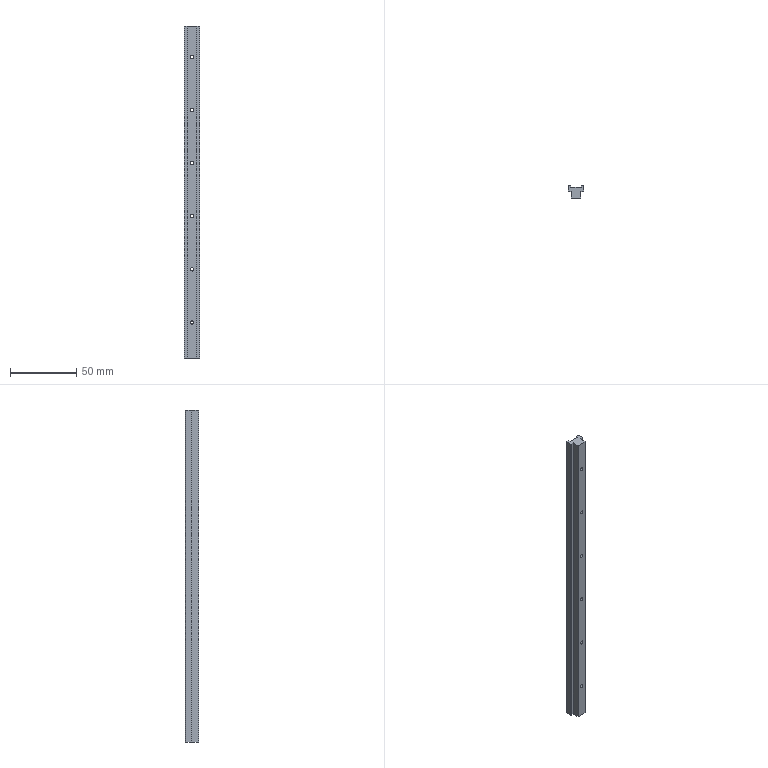Part | SolidWorks | features Chamfer 1, Extrusion 1, HoleWzd 1, LPattern 1 | 1 solid | 34 faces | box 12 x 10 x 250 mm | volume 20615 mm3 | plane 22 | cylinder 12 | commonest cylinder face diameters 2.5 x12
STEP:
#1=CARTESIAN_POINT('',(0.,-8.5,-59.5));
#2=VERTEX_POINT('',#1);
#3=CARTESIAN_POINT('',(0.,-8.5,-57.));
#4=VERTEX_POINT('',#3);
#5=CARTESIAN_POINT('',(0.,-8.5,-58.25));
#6=DIRECTION('',(0.,1.,0.));
#7=DIRECTION('',(0.,0.,1.));
#8=AXIS2_PLACEMENT_3D('',#5,#6,#7);
#9=CIRCLE('',#8,1.25);
#10=EDGE_CURVE('',#2,#4,#9,.T.);
#11=ORIENTED_EDGE('',*,*,#10,.F.);
#12=CARTESIAN_POINT('',(0.,0.,-59.5));
#13=VERTEX_POINT('',#12);
#14=CARTESIAN_POINT('',(0.,0.,-59.5));
#15=DIRECTION('',(0.,1.,0.));
#16=VECTOR('',#15,1000.);
#17=LINE('',#14,#16);
#18=EDGE_CURVE('',#2,#13,#17,.T.);
#19=ORIENTED_EDGE('',*,*,#18,.T.);
#20=CARTESIAN_POINT('',(0.,0.,-57.));
#21=VERTEX_POINT('',#20);
#22=CARTESIAN_POINT('',(0.,0.,-58.25));
#23=DIRECTION('',(0.,1.,0.));
#24=DIRECTION('',(0.,0.,1.));
#25=AXIS2_PLACEMENT_3D('',#22,#23,#24);
#26=CIRCLE('',#25,1.25);
#27=EDGE_CURVE('',#13,#21,#26,.T.);
#28=ORIENTED_EDGE('',*,*,#27,.T.);
#29=CARTESIAN_POINT('',(0.,0.,-57.));
#30=DIRECTION('',(0.,1.,0.));
#31=VECTOR('',#30,1000.);
#32=LINE('',#29,#31);
#33=EDGE_CURVE('',#4,#21,#32,.T.);
#34=ORIENTED_EDGE('',*,*,#33,.F.);
#35=EDGE_LOOP('',(#11,#19,#28,#34));
#36=FACE_OUTER_BOUND('',#35,.T.);
#37=CARTESIAN_POINT('',(0.,0.,-58.25));
#38=DIRECTION('',(0.,1.,0.));
#39=DIRECTION('',(0.,0.,1.));
#40=AXIS2_PLACEMENT_3D('',#37,#38,#39);
#41=CYLINDRICAL_SURFACE('',#40,1.25);
#42=ADVANCED_FACE('',(#36),#41,.F.);
#43=CARTESIAN_POINT('',(0.,-8.5,-99.5));
#44=VERTEX_POINT('',#43);
#45=CARTESIAN_POINT('',(0.,-8.5,-97.));
#46=VERTEX_POINT('',#45);
#47=CARTESIAN_POINT('',(0.,-8.5,-98.25));
#48=DIRECTION('',(0.,1.,0.));
#49=DIRECTION('',(0.,0.,1.));
#50=AXIS2_PLACEMENT_3D('',#47,#48,#49);
#51=CIRCLE('',#50,1.25);
#52=EDGE_CURVE('',#44,#46,#51,.T.);
#53=ORIENTED_EDGE('',*,*,#52,.F.);
#54=CARTESIAN_POINT('',(0.,0.,-99.5));
#55=VERTEX_POINT('',#54);
#56=CARTESIAN_POINT('',(0.,0.,-99.5));
#57=DIRECTION('',(0.,1.,0.));
#58=VECTOR('',#57,1000.);
#59=LINE('',#56,#58);
#60=EDGE_CURVE('',#44,#55,#59,.T.);
#61=ORIENTED_EDGE('',*,*,#60,.T.);
#62=CARTESIAN_POINT('',(0.,0.,-97.));
#63=VERTEX_POINT('',#62);
#64=CARTESIAN_POINT('',(0.,0.,-98.25));
#65=DIRECTION('',(0.,1.,0.));
#66=DIRECTION('',(0.,0.,1.));
#67=AXIS2_PLACEMENT_3D('',#64,#65,#66);
#68=CIRCLE('',#67,1.25);
#69=EDGE_CURVE('',#55,#63,#68,.T.);
#70=ORIENTED_EDGE('',*,*,#69,.T.);
#71=CARTESIAN_POINT('',(0.,0.,-97.));
#72=DIRECTION('',(0.,1.,0.));
#73=VECTOR('',#72,1000.);
#74=LINE('',#71,#73);
#75=EDGE_CURVE('',#46,#63,#74,.T.);
#76=ORIENTED_EDGE('',*,*,#75,.F.);
#77=EDGE_LOOP('',(#53,#61,#70,#76));
#78=FACE_OUTER_BOUND('',#77,.T.);
#79=CARTESIAN_POINT('',(0.,0.,-98.25));
#80=DIRECTION('',(0.,1.,0.));
#81=DIRECTION('',(0.,0.,1.));
#82=AXIS2_PLACEMENT_3D('',#79,#80,#81);
#83=CYLINDRICAL_SURFACE('',#82,1.25);
#84=ADVANCED_FACE('',(#78),#83,.F.);
#85=CARTESIAN_POINT('',(0.,-8.5,-19.5));
#86=VERTEX_POINT('',#85);
#87=CARTESIAN_POINT('',(0.,-8.5,-17.));
#88=VERTEX_POINT('',#87);
#89=CARTESIAN_POINT('',(0.,-8.5,-18.25));
#90=DIRECTION('',(0.,1.,0.));
#91=DIRECTION('',(0.,0.,1.));
#92=AXIS2_PLACEMENT_3D('',#89,#90,#91);
#93=CIRCLE('',#92,1.25);
#94=EDGE_CURVE('',#86,#88,#93,.T.);
#95=ORIENTED_EDGE('',*,*,#94,.F.);
#96=CARTESIAN_POINT('',(0.,0.,-19.5));
#97=VERTEX_POINT('',#96);
#98=CARTESIAN_POINT('',(0.,0.,-19.5));
#99=DIRECTION('',(0.,1.,0.));
#100=VECTOR('',#99,1000.);
#101=LINE('',#98,#100);
#102=EDGE_CURVE('',#86,#97,#101,.T.);
#103=ORIENTED_EDGE('',*,*,#102,.T.);
#104=CARTESIAN_POINT('',(0.,0.,-17.));
#105=VERTEX_POINT('',#104);
#106=CARTESIAN_POINT('',(0.,0.,-18.25));
#107=DIRECTION('',(0.,1.,0.));
#108=DIRECTION('',(0.,0.,1.));
#109=AXIS2_PLACEMENT_3D('',#106,#107,#108);
#110=CIRCLE('',#109,1.25);
#111=EDGE_CURVE('',#97,#105,#110,.T.);
#112=ORIENTED_EDGE('',*,*,#111,.T.);
#113=CARTESIAN_POINT('',(0.,0.,-17.));
#114=DIRECTION('',(0.,1.,0.));
#115=VECTOR('',#114,1000.);
#116=LINE('',#113,#115);
#117=EDGE_CURVE('',#88,#105,#116,.T.);
#118=ORIENTED_EDGE('',*,*,#117,.F.);
#119=EDGE_LOOP('',(#95,#103,#112,#118));
#120=FACE_OUTER_BOUND('',#119,.T.);
#121=CARTESIAN_POINT('',(0.,0.,-18.25));
#122=DIRECTION('',(0.,1.,0.));
#123=DIRECTION('',(0.,0.,1.));
#124=AXIS2_PLACEMENT_3D('',#121,#122,#123);
#125=CYLINDRICAL_SURFACE('',#124,1.25);
#126=ADVANCED_FACE('',(#120),#125,.F.);
#127=CARTESIAN_POINT('',(0.,-8.5,20.5));
#128=VERTEX_POINT('',#127);
#129=CARTESIAN_POINT('',(0.,-8.5,23.));
#130=VERTEX_POINT('',#129);
#131=CARTESIAN_POINT('',(0.,-8.5,21.75));
#132=DIRECTION('',(0.,1.,0.));
#133=DIRECTION('',(0.,0.,1.));
#134=AXIS2_PLACEMENT_3D('',#131,#132,#133);
#135=CIRCLE('',#134,1.25);
#136=EDGE_CURVE('',#128,#130,#135,.T.);
#137=ORIENTED_EDGE('',*,*,#136,.F.);
#138=CARTESIAN_POINT('',(0.,0.,20.5));
#139=VERTEX_POINT('',#138);
#140=CARTESIAN_POINT('',(0.,0.,20.5));
#141=DIRECTION('',(0.,1.,0.));
#142=VECTOR('',#141,1000.);
#143=LINE('',#140,#142);
#144=EDGE_CURVE('',#128,#139,#143,.T.);
#145=ORIENTED_EDGE('',*,*,#144,.T.);
#146=CARTESIAN_POINT('',(0.,0.,23.));
#147=VERTEX_POINT('',#146);
#148=CARTESIAN_POINT('',(0.,0.,21.75));
#149=DIRECTION('',(0.,1.,0.));
#150=DIRECTION('',(0.,0.,1.));
#151=AXIS2_PLACEMENT_3D('',#148,#149,#150);
#152=CIRCLE('',#151,1.25);
#153=EDGE_CURVE('',#139,#147,#152,.T.);
#154=ORIENTED_EDGE('',*,*,#153,.T.);
#155=CARTESIAN_POINT('',(0.,0.,23.));
#156=DIRECTION('',(0.,1.,0.));
#157=VECTOR('',#156,1000.);
#158=LINE('',#155,#157);
#159=EDGE_CURVE('',#130,#147,#158,.T.);
#160=ORIENTED_EDGE('',*,*,#159,.F.);
#161=EDGE_LOOP('',(#137,#145,#154,#160));
#162=FACE_OUTER_BOUND('',#161,.T.);
#163=CARTESIAN_POINT('',(0.,0.,21.75));
#164=DIRECTION('',(0.,1.,0.));
#165=DIRECTION('',(0.,0.,1.));
#166=AXIS2_PLACEMENT_3D('',#163,#164,#165);
#167=CYLINDRICAL_SURFACE('',#166,1.25);
#168=ADVANCED_FACE('',(#162),#167,.F.);
#169=CARTESIAN_POINT('',(0.,-8.5,60.5));
#170=VERTEX_POINT('',#169);
#171=CARTESIAN_POINT('',(0.,-8.5,63.));
#172=VERTEX_POINT('',#171);
#173=CARTESIAN_POINT('',(0.,-8.5,61.75));
#174=DIRECTION('',(0.,1.,0.));
#175=DIRECTION('',(0.,0.,1.));
#176=AXIS2_PLACEMENT_3D('',#173,#174,#175);
#177=CIRCLE('',#176,1.25);
#178=EDGE_CURVE('',#170,#172,#177,.T.);
#179=ORIENTED_EDGE('',*,*,#178,.F.);
#180=CARTESIAN_POINT('',(0.,0.,60.5));
#181=VERTEX_POINT('',#180);
#182=CARTESIAN_POINT('',(0.,0.,60.5));
#183=DIRECTION('',(0.,1.,0.));
#184=VECTOR('',#183,1000.);
#185=LINE('',#182,#184);
#186=EDGE_CURVE('',#170,#181,#185,.T.);
#187=ORIENTED_EDGE('',*,*,#186,.T.);
#188=CARTESIAN_POINT('',(0.,0.,63.));
#189=VERTEX_POINT('',#188);
#190=CARTESIAN_POINT('',(0.,0.,61.75));
#191=DIRECTION('',(0.,1.,0.));
#192=DIRECTION('',(0.,0.,1.));
#193=AXIS2_PLACEMENT_3D('',#190,#191,#192);
#194=CIRCLE('',#193,1.25);
#195=EDGE_CURVE('',#181,#189,#194,.T.);
#196=ORIENTED_EDGE('',*,*,#195,.T.);
#197=CARTESIAN_POINT('',(0.,0.,63.));
#198=DIRECTION('',(0.,1.,0.));
#199=VECTOR('',#198,1000.);
#200=LINE('',#197,#199);
#201=EDGE_CURVE('',#172,#189,#200,.T.);
#202=ORIENTED_EDGE('',*,*,#201,.F.);
#203=EDGE_LOOP('',(#179,#187,#196,#202));
#204=FACE_OUTER_BOUND('',#203,.T.);
#205=CARTESIAN_POINT('',(0.,0.,61.75));
#206=DIRECTION('',(0.,1.,0.));
#207=DIRECTION('',(0.,0.,1.));
#208=AXIS2_PLACEMENT_3D('',#205,#206,#207);
#209=CYLINDRICAL_SURFACE('',#208,1.25);
#210=ADVANCED_FACE('',(#204),#209,.F.);
#211=CARTESIAN_POINT('',(0.,-8.5,100.5));
#212=VERTEX_POINT('',#211);
#213=CARTESIAN_POINT('',(0.,-8.5,103.));
#214=VERTEX_POINT('',#213);
#215=CARTESIAN_POINT('',(0.,-8.5,101.75));
#216=DIRECTION('',(0.,1.,0.));
#217=DIRECTION('',(0.,0.,1.));
#218=AXIS2_PLACEMENT_3D('',#215,#216,#217);
#219=CIRCLE('',#218,1.25);
#220=EDGE_CURVE('',#212,#214,#219,.T.);
#221=ORIENTED_EDGE('',*,*,#220,.F.);
#222=CARTESIAN_POINT('',(0.,0.,100.5));
#223=VERTEX_POINT('',#222);
#224=CARTESIAN_POINT('',(0.,0.,100.5));
#225=DIRECTION('',(0.,1.,0.));
#226=VECTOR('',#225,1000.);
#227=LINE('',#224,#226);
#228=EDGE_CURVE('',#212,#223,#227,.T.);
#229=ORIENTED_EDGE('',*,*,#228,.T.);
#230=CARTESIAN_POINT('',(0.,0.,103.));
#231=VERTEX_POINT('',#230);
#232=CARTESIAN_POINT('',(0.,0.,101.75));
#233=DIRECTION('',(0.,1.,0.));
#234=DIRECTION('',(0.,0.,1.));
#235=AXIS2_PLACEMENT_3D('',#232,#233,#234);
#236=CIRCLE('',#235,1.25);
#237=EDGE_CURVE('',#223,#231,#236,.T.);
#238=ORIENTED_EDGE('',*,*,#237,.T.);
#239=CARTESIAN_POINT('',(0.,0.,103.));
#240=DIRECTION('',(0.,1.,0.));
#241=VECTOR('',#240,1000.);
#242=LINE('',#239,#241);
#243=EDGE_CURVE('',#214,#231,#242,.T.);
#244=ORIENTED_EDGE('',*,*,#243,.F.);
#245=EDGE_LOOP('',(#221,#229,#238,#244));
#246=FACE_OUTER_BOUND('',#245,.T.);
#247=CARTESIAN_POINT('',(0.,0.,101.75));
#248=DIRECTION('',(0.,1.,0.));
#249=DIRECTION('',(0.,0.,1.));
#250=AXIS2_PLACEMENT_3D('',#247,#248,#249);
#251=CYLINDRICAL_SURFACE('',#250,1.25);
#252=ADVANCED_FACE('',(#246),#251,.F.);
#253=ORIENTED_EDGE('',*,*,#228,.F.);
#254=CARTESIAN_POINT('',(0.,-8.5,101.75));
#255=DIRECTION('',(0.,1.,0.));
#256=DIRECTION('',(0.,0.,1.));
#257=AXIS2_PLACEMENT_3D('',#254,#255,#256);
#258=CIRCLE('',#257,1.25);
#259=EDGE_CURVE('',#214,#212,#258,.T.);
#260=ORIENTED_EDGE('',*,*,#259,.F.);
#261=ORIENTED_EDGE('',*,*,#243,.T.);
#262=CARTESIAN_POINT('',(0.,0.,101.75));
#263=DIRECTION('',(0.,1.,0.));
#264=DIRECTION('',(0.,0.,1.));
#265=AXIS2_PLACEMENT_3D('',#262,#263,#264);
#266=CIRCLE('',#265,1.25);
#267=EDGE_CURVE('',#231,#223,#266,.T.);
#268=ORIENTED_EDGE('',*,*,#267,.T.);
#269=EDGE_LOOP('',(#253,#260,#261,#268));
#270=FACE_OUTER_BOUND('',#269,.T.);
#271=CARTESIAN_POINT('',(0.,0.,101.75));
#272=DIRECTION('',(0.,1.,0.));
#273=DIRECTION('',(0.,0.,1.));
#274=AXIS2_PLACEMENT_3D('',#271,#272,#273);
#275=CYLINDRICAL_SURFACE('',#274,1.25);
#276=ADVANCED_FACE('',(#270),#275,.F.);
#277=ORIENTED_EDGE('',*,*,#186,.F.);
#278=CARTESIAN_POINT('',(0.,-8.5,61.75));
#279=DIRECTION('',(0.,1.,0.));
#280=DIRECTION('',(0.,0.,1.));
#281=AXIS2_PLACEMENT_3D('',#278,#279,#280);
#282=CIRCLE('',#281,1.25);
#283=EDGE_CURVE('',#172,#170,#282,.T.);
#284=ORIENTED_EDGE('',*,*,#283,.F.);
#285=ORIENTED_EDGE('',*,*,#201,.T.);
#286=CARTESIAN_POINT('',(0.,0.,61.75));
#287=DIRECTION('',(0.,1.,0.));
#288=DIRECTION('',(0.,0.,1.));
#289=AXIS2_PLACEMENT_3D('',#286,#287,#288);
#290=CIRCLE('',#289,1.25);
#291=EDGE_CURVE('',#189,#181,#290,.T.);
#292=ORIENTED_EDGE('',*,*,#291,.T.);
#293=EDGE_LOOP('',(#277,#284,#285,#292));
#294=FACE_OUTER_BOUND('',#293,.T.);
#295=CARTESIAN_POINT('',(0.,0.,61.75));
#296=DIRECTION('',(0.,1.,0.));
#297=DIRECTION('',(0.,0.,1.));
#298=AXIS2_PLACEMENT_3D('',#295,#296,#297);
#299=CYLINDRICAL_SURFACE('',#298,1.25);
#300=ADVANCED_FACE('',(#294),#299,.F.);
#301=ORIENTED_EDGE('',*,*,#144,.F.);
#302=CARTESIAN_POINT('',(0.,-8.5,21.75));
#303=DIRECTION('',(0.,1.,0.));
#304=DIRECTION('',(0.,0.,1.));
#305=AXIS2_PLACEMENT_3D('',#302,#303,#304);
#306=CIRCLE('',#305,1.25);
#307=EDGE_CURVE('',#130,#128,#306,.T.);
#308=ORIENTED_EDGE('',*,*,#307,.F.);
#309=ORIENTED_EDGE('',*,*,#159,.T.);
#310=CARTESIAN_POINT('',(0.,0.,21.75));
#311=DIRECTION('',(0.,1.,0.));
#312=DIRECTION('',(0.,0.,1.));
#313=AXIS2_PLACEMENT_3D('',#310,#311,#312);
#314=CIRCLE('',#313,1.25);
#315=EDGE_CURVE('',#147,#139,#314,.T.);
#316=ORIENTED_EDGE('',*,*,#315,.T.);
#317=EDGE_LOOP('',(#301,#308,#309,#316));
#318=FACE_OUTER_BOUND('',#317,.T.);
#319=CARTESIAN_POINT('',(0.,0.,21.75));
#320=DIRECTION('',(0.,1.,0.));
#321=DIRECTION('',(0.,0.,1.));
#322=AXIS2_PLACEMENT_3D('',#319,#320,#321);
#323=CYLINDRICAL_SURFACE('',#322,1.25);
#324=ADVANCED_FACE('',(#318),#323,.F.);
#325=ORIENTED_EDGE('',*,*,#102,.F.);
#326=CARTESIAN_POINT('',(0.,-8.5,-18.25));
#327=DIRECTION('',(0.,1.,0.));
#328=DIRECTION('',(0.,0.,1.));
#329=AXIS2_PLACEMENT_3D('',#326,#327,#328);
#330=CIRCLE('',#329,1.25);
#331=EDGE_CURVE('',#88,#86,#330,.T.);
#332=ORIENTED_EDGE('',*,*,#331,.F.);
#333=ORIENTED_EDGE('',*,*,#117,.T.);
#334=CARTESIAN_POINT('',(0.,0.,-18.25));
#335=DIRECTION('',(0.,1.,0.));
#336=DIRECTION('',(0.,0.,1.));
#337=AXIS2_PLACEMENT_3D('',#334,#335,#336);
#338=CIRCLE('',#337,1.25);
#339=EDGE_CURVE('',#105,#97,#338,.T.);
#340=ORIENTED_EDGE('',*,*,#339,.T.);
#341=EDGE_LOOP('',(#325,#332,#333,#340));
#342=FACE_OUTER_BOUND('',#341,.T.);
#343=CARTESIAN_POINT('',(0.,0.,-18.25));
#344=DIRECTION('',(0.,1.,0.));
#345=DIRECTION('',(0.,0.,1.));
#346=AXIS2_PLACEMENT_3D('',#343,#344,#345);
#347=CYLINDRICAL_SURFACE('',#346,1.25);
#348=ADVANCED_FACE('',(#342),#347,.F.);
#349=CARTESIAN_POINT('',(-4.,0.,-125.));
#350=VERTEX_POINT('',#349);
#351=CARTESIAN_POINT('',(-4.,1.3,-125.));
#352=VERTEX_POINT('',#351);
#353=CARTESIAN_POINT('',(-4.,0.,-125.));
#354=DIRECTION('',(0.,1.,0.));
#355=VECTOR('',#354,1000.);
#356=LINE('',#353,#355);
#357=EDGE_CURVE('',#350,#352,#356,.T.);
#358=ORIENTED_EDGE('',*,*,#357,.T.);
#359=CARTESIAN_POINT('',(-4.,1.3,125.));
#360=VERTEX_POINT('',#359);
#361=CARTESIAN_POINT('',(-4.,1.3,125.));
#362=DIRECTION('',(0.,0.,1.));
#363=VECTOR('',#362,1000.);
#364=LINE('',#361,#363);
#365=EDGE_CURVE('',#352,#360,#364,.T.);
#366=ORIENTED_EDGE('',*,*,#365,.T.);
#367=CARTESIAN_POINT('',(-4.,0.,125.));
#368=VERTEX_POINT('',#367);
#369=CARTESIAN_POINT('',(-4.,0.,125.));
#370=DIRECTION('',(0.,1.,0.));
#371=VECTOR('',#370,1000.);
#372=LINE('',#369,#371);
#373=EDGE_CURVE('',#368,#360,#372,.T.);
#374=ORIENTED_EDGE('',*,*,#373,.F.);
#375=CARTESIAN_POINT('',(-4.,0.,125.));
#376=DIRECTION('',(0.,0.,-1.));
#377=VECTOR('',#376,1000.);
#378=LINE('',#375,#377);
#379=EDGE_CURVE('',#368,#350,#378,.T.);
#380=ORIENTED_EDGE('',*,*,#379,.T.);
#381=EDGE_LOOP('',(#358,#366,#374,#380));
#382=FACE_OUTER_BOUND('',#381,.T.);
#383=CARTESIAN_POINT('',(-4.,0.,125.));
#384=DIRECTION('',(-1.,0.,0.));
#385=DIRECTION('',(0.,-1.,0.));
#386=AXIS2_PLACEMENT_3D('',#383,#384,#385);
#387=PLANE('',#386);
#388=ADVANCED_FACE('',(#382),#387,.F.);
#389=CARTESIAN_POINT('',(-4.2,1.5,-125.));
#390=VERTEX_POINT('',#389);
#391=CARTESIAN_POINT('',(-5.8,1.5,-125.));
#392=VERTEX_POINT('',#391);
#393=CARTESIAN_POINT('',(-4.,1.5,-125.));
#394=DIRECTION('',(-1.,0.,0.));
#395=VECTOR('',#394,1000.);
#396=LINE('',#393,#395);
#397=EDGE_CURVE('',#390,#392,#396,.T.);
#398=ORIENTED_EDGE('',*,*,#397,.T.);
#399=CARTESIAN_POINT('',(-5.8,1.5,125.));
#400=VERTEX_POINT('',#399);
#401=CARTESIAN_POINT('',(-5.8,1.5,125.));
#402=DIRECTION('',(0.,0.,1.));
#403=VECTOR('',#402,1000.);
#404=LINE('',#401,#403);
#405=EDGE_CURVE('',#392,#400,#404,.T.);
#406=ORIENTED_EDGE('',*,*,#405,.T.);
#407=CARTESIAN_POINT('',(-4.2,1.5,125.));
#408=VERTEX_POINT('',#407);
#409=CARTESIAN_POINT('',(-4.,1.5,125.));
#410=DIRECTION('',(-1.,0.,0.));
#411=VECTOR('',#410,1000.);
#412=LINE('',#409,#411);
#413=EDGE_CURVE('',#408,#400,#412,.T.);
#414=ORIENTED_EDGE('',*,*,#413,.F.);
#415=CARTESIAN_POINT('',(-4.2,1.5,125.));
#416=DIRECTION('',(0.,0.,-1.));
#417=VECTOR('',#416,1000.);
#418=LINE('',#415,#417);
#419=EDGE_CURVE('',#408,#390,#418,.T.);
#420=ORIENTED_EDGE('',*,*,#419,.T.);
#421=EDGE_LOOP('',(#398,#406,#414,#420));
#422=FACE_OUTER_BOUND('',#421,.T.);
#423=CARTESIAN_POINT('',(-4.,1.5,125.));
#424=DIRECTION('',(0.,-1.,0.));
#425=DIRECTION('',(0.,0.,-1.));
#426=AXIS2_PLACEMENT_3D('',#423,#424,#425);
#427=PLANE('',#426);
#428=ADVANCED_FACE('',(#422),#427,.F.);
#429=CARTESIAN_POINT('',(-6.,1.3,125.));
#430=VERTEX_POINT('',#429);
#431=CARTESIAN_POINT('',(-6.,-3.,125.));
#432=VERTEX_POINT('',#431);
#433=CARTESIAN_POINT('',(-6.,1.5,125.));
#434=DIRECTION('',(0.,-1.,0.));
#435=VECTOR('',#434,1000.);
#436=LINE('',#433,#435);
#437=EDGE_CURVE('',#430,#432,#436,.T.);
#438=ORIENTED_EDGE('',*,*,#437,.F.);
#439=CARTESIAN_POINT('',(-6.,1.3,-125.));
#440=VERTEX_POINT('',#439);
#441=CARTESIAN_POINT('',(-6.,1.3,125.));
#442=DIRECTION('',(0.,0.,-1.));
#443=VECTOR('',#442,1000.);
#444=LINE('',#441,#443);
#445=EDGE_CURVE('',#430,#440,#444,.T.);
#446=ORIENTED_EDGE('',*,*,#445,.T.);
#447=CARTESIAN_POINT('',(-6.,-3.,-125.));
#448=VERTEX_POINT('',#447);
#449=CARTESIAN_POINT('',(-6.,1.5,-125.));
#450=DIRECTION('',(0.,-1.,0.));
#451=VECTOR('',#450,1000.);
#452=LINE('',#449,#451);
#453=EDGE_CURVE('',#440,#448,#452,.T.);
#454=ORIENTED_EDGE('',*,*,#453,.T.);
#455=CARTESIAN_POINT('',(-6.,-3.,125.));
#456=DIRECTION('',(0.,0.,1.));
#457=VECTOR('',#456,1000.);
#458=LINE('',#455,#457);
#459=EDGE_CURVE('',#448,#432,#458,.T.);
#460=ORIENTED_EDGE('',*,*,#459,.T.);
#461=EDGE_LOOP('',(#438,#446,#454,#460));
#462=FACE_OUTER_BOUND('',#461,.T.);
#463=CARTESIAN_POINT('',(-6.,1.5,125.));
#464=DIRECTION('',(1.,0.,0.));
#465=DIRECTION('',(0.,1.,0.));
#466=AXIS2_PLACEMENT_3D('',#463,#464,#465);
#467=PLANE('',#466);
#468=ADVANCED_FACE('',(#462),#467,.F.);
#469=CARTESIAN_POINT('',(-5.8,-3.2,125.));
#470=VERTEX_POINT('',#469);
#471=CARTESIAN_POINT('',(-3.7,-3.2,125.));
#472=VERTEX_POINT('',#471);
#473=CARTESIAN_POINT('',(-6.,-3.2,125.));
#474=DIRECTION('',(1.,0.,0.));
#475=VECTOR('',#474,1000.);
#476=LINE('',#473,#475);
#477=EDGE_CURVE('',#470,#472,#476,.T.);
#478=ORIENTED_EDGE('',*,*,#477,.F.);
#479=CARTESIAN_POINT('',(-5.8,-3.2,-125.));
#480=VERTEX_POINT('',#479);
#481=CARTESIAN_POINT('',(-5.8,-3.2,125.));
#482=DIRECTION('',(0.,0.,-1.));
#483=VECTOR('',#482,1000.);
#484=LINE('',#481,#483);
#485=EDGE_CURVE('',#470,#480,#484,.T.);
#486=ORIENTED_EDGE('',*,*,#485,.T.);
#487=CARTESIAN_POINT('',(-3.7,-3.2,-125.));
#488=VERTEX_POINT('',#487);
#489=CARTESIAN_POINT('',(-6.,-3.2,-125.));
#490=DIRECTION('',(1.,0.,0.));
#491=VECTOR('',#490,1000.);
#492=LINE('',#489,#491);
#493=EDGE_CURVE('',#480,#488,#492,.T.);
#494=ORIENTED_EDGE('',*,*,#493,.T.);
#495=CARTESIAN_POINT('',(-3.7,-3.2,125.));
#496=DIRECTION('',(0.,0.,-1.));
#497=VECTOR('',#496,1000.);
#498=LINE('',#495,#497);
#499=EDGE_CURVE('',#472,#488,#498,.T.);
#500=ORIENTED_EDGE('',*,*,#499,.F.);
#501=EDGE_LOOP('',(#478,#486,#494,#500));
#502=FACE_OUTER_BOUND('',#501,.T.);
#503=CARTESIAN_POINT('',(-6.,-3.2,125.));
#504=DIRECTION('',(0.,1.,0.));
#505=DIRECTION('',(0.,0.,1.));
#506=AXIS2_PLACEMENT_3D('',#503,#504,#505);
#507=PLANE('',#506);
#508=ADVANCED_FACE('',(#502),#507,.F.);
#509=CARTESIAN_POINT('',(-3.7,-8.3,-125.));
#510=VERTEX_POINT('',#509);
#511=CARTESIAN_POINT('',(-3.7,-3.2,-125.));
#512=DIRECTION('',(0.,-1.,0.));
#513=VECTOR('',#512,1000.);
#514=LINE('',#511,#513);
#515=EDGE_CURVE('',#488,#510,#514,.T.);
#516=ORIENTED_EDGE('',*,*,#515,.T.);
#517=CARTESIAN_POINT('',(-3.7,-8.3,125.));
#518=VERTEX_POINT('',#517);
#519=CARTESIAN_POINT('',(-3.7,-8.3,125.));
#520=DIRECTION('',(0.,0.,1.));
#521=VECTOR('',#520,1000.);
#522=LINE('',#519,#521);
#523=EDGE_CURVE('',#510,#518,#522,.T.);
#524=ORIENTED_EDGE('',*,*,#523,.T.);
#525=CARTESIAN_POINT('',(-3.7,-3.2,125.));
#526=DIRECTION('',(0.,-1.,0.));
#527=VECTOR('',#526,1000.);
#528=LINE('',#525,#527);
#529=EDGE_CURVE('',#472,#518,#528,.T.);
#530=ORIENTED_EDGE('',*,*,#529,.F.);
#531=ORIENTED_EDGE('',*,*,#499,.T.);
#532=EDGE_LOOP('',(#516,#524,#530,#531));
#533=FACE_OUTER_BOUND('',#532,.T.);
#534=CARTESIAN_POINT('',(-3.7,-3.2,125.));
#535=DIRECTION('',(1.,0.,0.));
#536=DIRECTION('',(0.,1.,0.));
#537=AXIS2_PLACEMENT_3D('',#534,#535,#536);
#538=PLANE('',#537);
#539=ADVANCED_FACE('',(#533),#538,.F.);
#540=CARTESIAN_POINT('',(0.,-8.5,-58.25));
#541=DIRECTION('',(0.,1.,0.));
#542=DIRECTION('',(0.,0.,1.));
#543=AXIS2_PLACEMENT_3D('',#540,#541,#542);
#544=CIRCLE('',#543,1.25);
#545=EDGE_CURVE('',#4,#2,#544,.T.);
#546=ORIENTED_EDGE('',*,*,#545,.T.);
#547=ORIENTED_EDGE('',*,*,#10,.T.);
#548=EDGE_LOOP('',(#546,#547));
#549=FACE_BOUND('',#548,.T.);
#550=CARTESIAN_POINT('',(0.,-8.5,-98.25));
#551=DIRECTION('',(0.,1.,0.));
#552=DIRECTION('',(0.,0.,1.));
#553=AXIS2_PLACEMENT_3D('',#550,#551,#552);
#554=CIRCLE('',#553,1.25);
#555=EDGE_CURVE('',#46,#44,#554,.T.);
#556=ORIENTED_EDGE('',*,*,#555,.T.);
#557=ORIENTED_EDGE('',*,*,#52,.T.);
#558=EDGE_LOOP('',(#556,#557));
#559=FACE_BOUND('',#558,.T.);
#560=CARTESIAN_POINT('',(-3.5,-8.5,125.));
#561=VERTEX_POINT('',#560);
#562=CARTESIAN_POINT('',(3.5,-8.5,125.));
#563=VERTEX_POINT('',#562);
#564=CARTESIAN_POINT('',(-3.7,-8.5,125.));
#565=DIRECTION('',(1.,0.,0.));
#566=VECTOR('',#565,1000.);
#567=LINE('',#564,#566);
#568=EDGE_CURVE('',#561,#563,#567,.T.);
#569=ORIENTED_EDGE('',*,*,#568,.F.);
#570=CARTESIAN_POINT('',(-3.5,-8.5,-125.));
#571=VERTEX_POINT('',#570);
#572=CARTESIAN_POINT('',(-3.5,-8.5,125.));
#573=DIRECTION('',(0.,0.,-1.));
#574=VECTOR('',#573,1000.);
#575=LINE('',#572,#574);
#576=EDGE_CURVE('',#561,#571,#575,.T.);
#577=ORIENTED_EDGE('',*,*,#576,.T.);
#578=CARTESIAN_POINT('',(3.5,-8.5,-125.));
#579=VERTEX_POINT('',#578);
#580=CARTESIAN_POINT('',(-3.7,-8.5,-125.));
#581=DIRECTION('',(1.,0.,0.));
#582=VECTOR('',#581,1000.);
#583=LINE('',#580,#582);
#584=EDGE_CURVE('',#571,#579,#583,.T.);
#585=ORIENTED_EDGE('',*,*,#584,.T.);
#586=CARTESIAN_POINT('',(3.5,-8.5,125.));
#587=DIRECTION('',(0.,0.,1.));
#588=VECTOR('',#587,1000.);
#589=LINE('',#586,#588);
#590=EDGE_CURVE('',#579,#563,#589,.T.);
#591=ORIENTED_EDGE('',*,*,#590,.T.);
#592=EDGE_LOOP('',(#569,#577,#585,#591));
#593=FACE_OUTER_BOUND('',#592,.T.);
#594=ORIENTED_EDGE('',*,*,#331,.T.);
#595=ORIENTED_EDGE('',*,*,#94,.T.);
#596=EDGE_LOOP('',(#594,#595));
#597=FACE_BOUND('',#596,.T.);
#598=ORIENTED_EDGE('',*,*,#307,.T.);
#599=ORIENTED_EDGE('',*,*,#136,.T.);
#600=EDGE_LOOP('',(#598,#599));
#601=FACE_BOUND('',#600,.T.);
#602=ORIENTED_EDGE('',*,*,#283,.T.);
#603=ORIENTED_EDGE('',*,*,#178,.T.);
#604=EDGE_LOOP('',(#602,#603));
#605=FACE_BOUND('',#604,.T.);
#606=ORIENTED_EDGE('',*,*,#259,.T.);
#607=ORIENTED_EDGE('',*,*,#220,.T.);
#608=EDGE_LOOP('',(#606,#607));
#609=FACE_BOUND('',#608,.T.);
#610=CARTESIAN_POINT('',(-3.7,-8.5,125.));
#611=DIRECTION('',(0.,1.,0.));
#612=DIRECTION('',(0.,0.,1.));
#613=AXIS2_PLACEMENT_3D('',#610,#611,#612);
#614=PLANE('',#613);
#615=ADVANCED_FACE('',(#549,#559,#593,#597,#601,#605,#609),#614,.F.);
#616=CARTESIAN_POINT('',(3.7,-8.3,125.));
#617=VERTEX_POINT('',#616);
#618=CARTESIAN_POINT('',(3.7,-3.2,125.));
#619=VERTEX_POINT('',#618);
#620=CARTESIAN_POINT('',(3.7,-3.2,125.));
#621=DIRECTION('',(0.,1.,0.));
#622=VECTOR('',#621,1000.);
#623=LINE('',#620,#622);
#624=EDGE_CURVE('',#617,#619,#623,.T.);
#625=ORIENTED_EDGE('',*,*,#624,.F.);
#626=CARTESIAN_POINT('',(3.7,-8.3,-125.));
#627=VERTEX_POINT('',#626);
#628=CARTESIAN_POINT('',(3.7,-8.3,125.));
#629=DIRECTION('',(0.,0.,-1.));
#630=VECTOR('',#629,1000.);
#631=LINE('',#628,#630);
#632=EDGE_CURVE('',#617,#627,#631,.T.);
#633=ORIENTED_EDGE('',*,*,#632,.T.);
#634=CARTESIAN_POINT('',(3.7,-3.2,-125.));
#635=VERTEX_POINT('',#634);
#636=CARTESIAN_POINT('',(3.7,-3.2,-125.));
#637=DIRECTION('',(0.,1.,0.));
#638=VECTOR('',#637,1000.);
#639=LINE('',#636,#638);
#640=EDGE_CURVE('',#627,#635,#639,.T.);
#641=ORIENTED_EDGE('',*,*,#640,.T.);
#642=CARTESIAN_POINT('',(3.7,-3.2,125.));
#643=DIRECTION('',(0.,0.,-1.));
#644=VECTOR('',#643,1000.);
#645=LINE('',#642,#644);
#646=EDGE_CURVE('',#619,#635,#645,.T.);
#647=ORIENTED_EDGE('',*,*,#646,.F.);
#648=EDGE_LOOP('',(#625,#633,#641,#647));
#649=FACE_OUTER_BOUND('',#648,.T.);
#650=CARTESIAN_POINT('',(3.7,-3.2,125.));
#651=DIRECTION('',(-1.,0.,0.));
#652=DIRECTION('',(0.,-1.,0.));
#653=AXIS2_PLACEMENT_3D('',#650,#651,#652);
#654=PLANE('',#653);
#655=ADVANCED_FACE('',(#649),#654,.F.);
#656=CARTESIAN_POINT('',(5.8,-3.2,-125.));
#657=VERTEX_POINT('',#656);
#658=CARTESIAN_POINT('',(6.,-3.2,-125.));
#659=DIRECTION('',(1.,0.,0.));
#660=VECTOR('',#659,1000.);
#661=LINE('',#658,#660);
#662=EDGE_CURVE('',#635,#657,#661,.T.);
#663=ORIENTED_EDGE('',*,*,#662,.T.);
#664=CARTESIAN_POINT('',(5.8,-3.2,125.));
#665=VERTEX_POINT('',#664);
#666=CARTESIAN_POINT('',(5.8,-3.2,125.));
#667=DIRECTION('',(0.,0.,1.));
#668=VECTOR('',#667,1000.);
#669=LINE('',#666,#668);
#670=EDGE_CURVE('',#657,#665,#669,.T.);
#671=ORIENTED_EDGE('',*,*,#670,.T.);
#672=CARTESIAN_POINT('',(6.,-3.2,125.));
#673=DIRECTION('',(1.,0.,0.));
#674=VECTOR('',#673,1000.);
#675=LINE('',#672,#674);
#676=EDGE_CURVE('',#619,#665,#675,.T.);
#677=ORIENTED_EDGE('',*,*,#676,.F.);
#678=ORIENTED_EDGE('',*,*,#646,.T.);
#679=EDGE_LOOP('',(#663,#671,#677,#678));
#680=FACE_OUTER_BOUND('',#679,.T.);
#681=CARTESIAN_POINT('',(6.,-3.2,125.));
#682=DIRECTION('',(0.,1.,0.));
#683=DIRECTION('',(0.,0.,1.));
#684=AXIS2_PLACEMENT_3D('',#681,#682,#683);
#685=PLANE('',#684);
#686=ADVANCED_FACE('',(#680),#685,.F.);
#687=CARTESIAN_POINT('',(6.,-3.,125.));
#688=VERTEX_POINT('',#687);
#689=CARTESIAN_POINT('',(6.,1.3,125.));
#690=VERTEX_POINT('',#689);
#691=CARTESIAN_POINT('',(6.,1.5,125.));
#692=DIRECTION('',(0.,1.,0.));
#693=VECTOR('',#692,1000.);
#694=LINE('',#691,#693);
#695=EDGE_CURVE('',#688,#690,#694,.T.);
#696=ORIENTED_EDGE('',*,*,#695,.F.);
#697=CARTESIAN_POINT('',(6.,-3.,-125.));
#698=VERTEX_POINT('',#697);
#699=CARTESIAN_POINT('',(6.,-3.,125.));
#700=DIRECTION('',(0.,0.,-1.));
#701=VECTOR('',#700,1000.);
#702=LINE('',#699,#701);
#703=EDGE_CURVE('',#688,#698,#702,.T.);
#704=ORIENTED_EDGE('',*,*,#703,.T.);
#705=CARTESIAN_POINT('',(6.,1.3,-125.));
#706=VERTEX_POINT('',#705);
#707=CARTESIAN_POINT('',(6.,1.5,-125.));
#708=DIRECTION('',(0.,1.,0.));
#709=VECTOR('',#708,1000.);
#710=LINE('',#707,#709);
#711=EDGE_CURVE('',#698,#706,#710,.T.);
#712=ORIENTED_EDGE('',*,*,#711,.T.);
#713=CARTESIAN_POINT('',(6.,1.3,125.));
#714=DIRECTION('',(0.,0.,1.));
#715=VECTOR('',#714,1000.);
#716=LINE('',#713,#715);
#717=EDGE_CURVE('',#706,#690,#716,.T.);
#718=ORIENTED_EDGE('',*,*,#717,.T.);
#719=EDGE_LOOP('',(#696,#704,#712,#718));
#720=FACE_OUTER_BOUND('',#719,.T.);
#721=CARTESIAN_POINT('',(6.,1.5,125.));
#722=DIRECTION('',(-1.,0.,0.));
#723=DIRECTION('',(0.,-1.,0.));
#724=AXIS2_PLACEMENT_3D('',#721,#722,#723);
#725=PLANE('',#724);
#726=ADVANCED_FACE('',(#720),#725,.F.);
#727=CARTESIAN_POINT('',(5.8,1.5,125.));
#728=VERTEX_POINT('',#727);
#729=CARTESIAN_POINT('',(4.2,1.5,125.));
#730=VERTEX_POINT('',#729);
#731=CARTESIAN_POINT('',(4.,1.5,125.));
#732=DIRECTION('',(-1.,0.,0.));
#733=VECTOR('',#732,1000.);
#734=LINE('',#731,#733);
#735=EDGE_CURVE('',#728,#730,#734,.T.);
#736=ORIENTED_EDGE('',*,*,#735,.F.);
#737=CARTESIAN_POINT('',(5.8,1.5,-125.));
#738=VERTEX_POINT('',#737);
#739=CARTESIAN_POINT('',(5.8,1.5,125.));
#740=DIRECTION('',(0.,0.,-1.));
#741=VECTOR('',#740,1000.);
#742=LINE('',#739,#741);
#743=EDGE_CURVE('',#728,#738,#742,.T.);
#744=ORIENTED_EDGE('',*,*,#743,.T.);
#745=CARTESIAN_POINT('',(4.2,1.5,-125.));
#746=VERTEX_POINT('',#745);
#747=CARTESIAN_POINT('',(4.,1.5,-125.));
#748=DIRECTION('',(-1.,0.,0.));
#749=VECTOR('',#748,1000.);
#750=LINE('',#747,#749);
#751=EDGE_CURVE('',#738,#746,#750,.T.);
#752=ORIENTED_EDGE('',*,*,#751,.T.);
#753=CARTESIAN_POINT('',(4.2,1.5,125.));
#754=DIRECTION('',(0.,0.,1.));
#755=VECTOR('',#754,1000.);
#756=LINE('',#753,#755);
#757=EDGE_CURVE('',#746,#730,#756,.T.);
#758=ORIENTED_EDGE('',*,*,#757,.T.);
#759=EDGE_LOOP('',(#736,#744,#752,#758));
#760=FACE_OUTER_BOUND('',#759,.T.);
#761=CARTESIAN_POINT('',(4.,1.5,125.));
#762=DIRECTION('',(0.,-1.,0.));
#763=DIRECTION('',(0.,0.,-1.));
#764=AXIS2_PLACEMENT_3D('',#761,#762,#763);
#765=PLANE('',#764);
#766=ADVANCED_FACE('',(#760),#765,.F.);
#767=CARTESIAN_POINT('',(4.,1.3,125.));
#768=VERTEX_POINT('',#767);
#769=CARTESIAN_POINT('',(4.,0.,125.));
#770=VERTEX_POINT('',#769);
#771=CARTESIAN_POINT('',(4.,0.,125.));
#772=DIRECTION('',(0.,-1.,0.));
#773=VECTOR('',#772,1000.);
#774=LINE('',#771,#773);
#775=EDGE_CURVE('',#768,#770,#774,.T.);
#776=ORIENTED_EDGE('',*,*,#775,.F.);
#777=CARTESIAN_POINT('',(4.,1.3,-125.));
#778=VERTEX_POINT('',#777);
#779=CARTESIAN_POINT('',(4.,1.3,125.));
#780=DIRECTION('',(0.,0.,-1.));
#781=VECTOR('',#780,1000.);
#782=LINE('',#779,#781);
#783=EDGE_CURVE('',#768,#778,#782,.T.);
#784=ORIENTED_EDGE('',*,*,#783,.T.);
#785=CARTESIAN_POINT('',(4.,0.,-125.));
#786=VERTEX_POINT('',#785);
#787=CARTESIAN_POINT('',(4.,0.,-125.));
#788=DIRECTION('',(0.,-1.,0.));
#789=VECTOR('',#788,1000.);
#790=LINE('',#787,#789);
#791=EDGE_CURVE('',#778,#786,#790,.T.);
#792=ORIENTED_EDGE('',*,*,#791,.T.);
#793=CARTESIAN_POINT('',(4.,0.,125.));
#794=DIRECTION('',(0.,0.,-1.));
#795=VECTOR('',#794,1000.);
#796=LINE('',#793,#795);
#797=EDGE_CURVE('',#770,#786,#796,.T.);
#798=ORIENTED_EDGE('',*,*,#797,.F.);
#799=EDGE_LOOP('',(#776,#784,#792,#798));
#800=FACE_OUTER_BOUND('',#799,.T.);
#801=CARTESIAN_POINT('',(4.,0.,125.));
#802=DIRECTION('',(1.,0.,0.));
#803=DIRECTION('',(0.,1.,0.));
#804=AXIS2_PLACEMENT_3D('',#801,#802,#803);
#805=PLANE('',#804);
#806=ADVANCED_FACE('',(#800),#805,.F.);
#807=CARTESIAN_POINT('',(0.,0.,-58.25));
#808=DIRECTION('',(0.,1.,0.));
#809=DIRECTION('',(0.,0.,1.));
#810=AXIS2_PLACEMENT_3D('',#807,#808,#809);
#811=CIRCLE('',#810,1.25);
#812=EDGE_CURVE('',#21,#13,#811,.T.);
#813=ORIENTED_EDGE('',*,*,#812,.F.);
#814=ORIENTED_EDGE('',*,*,#27,.F.);
#815=EDGE_LOOP('',(#813,#814));
#816=FACE_BOUND('',#815,.T.);
#817=CARTESIAN_POINT('',(0.,0.,-98.25));
#818=DIRECTION('',(0.,1.,0.));
#819=DIRECTION('',(0.,0.,1.));
#820=AXIS2_PLACEMENT_3D('',#817,#818,#819);
#821=CIRCLE('',#820,1.25);
#822=EDGE_CURVE('',#63,#55,#821,.T.);
#823=ORIENTED_EDGE('',*,*,#822,.F.);
#824=ORIENTED_EDGE('',*,*,#69,.F.);
#825=EDGE_LOOP('',(#823,#824));
#826=FACE_BOUND('',#825,.T.);
#827=CARTESIAN_POINT('',(4.,0.,-125.));
#828=DIRECTION('',(-1.,0.,0.));
#829=VECTOR('',#828,1000.);
#830=LINE('',#827,#829);
#831=EDGE_CURVE('',#786,#350,#830,.T.);
#832=ORIENTED_EDGE('',*,*,#831,.T.);
#833=ORIENTED_EDGE('',*,*,#379,.F.);
#834=CARTESIAN_POINT('',(4.,0.,125.));
#835=DIRECTION('',(-1.,0.,0.));
#836=VECTOR('',#835,1000.);
#837=LINE('',#834,#836);
#838=EDGE_CURVE('',#770,#368,#837,.T.);
#839=ORIENTED_EDGE('',*,*,#838,.F.);
#840=ORIENTED_EDGE('',*,*,#797,.T.);
#841=EDGE_LOOP('',(#832,#833,#839,#840));
#842=FACE_OUTER_BOUND('',#841,.T.);
#843=ORIENTED_EDGE('',*,*,#339,.F.);
#844=ORIENTED_EDGE('',*,*,#111,.F.);
#845=EDGE_LOOP('',(#843,#844));
#846=FACE_BOUND('',#845,.T.);
#847=ORIENTED_EDGE('',*,*,#315,.F.);
#848=ORIENTED_EDGE('',*,*,#153,.F.);
#849=EDGE_LOOP('',(#847,#848));
#850=FACE_BOUND('',#849,.T.);
#851=ORIENTED_EDGE('',*,*,#291,.F.);
#852=ORIENTED_EDGE('',*,*,#195,.F.);
#853=EDGE_LOOP('',(#851,#852));
#854=FACE_BOUND('',#853,.T.);
#855=ORIENTED_EDGE('',*,*,#267,.F.);
#856=ORIENTED_EDGE('',*,*,#237,.F.);
#857=EDGE_LOOP('',(#855,#856));
#858=FACE_BOUND('',#857,.T.);
#859=CARTESIAN_POINT('',(4.,0.,125.));
#860=DIRECTION('',(0.,-1.,0.));
#861=DIRECTION('',(0.,0.,-1.));
#862=AXIS2_PLACEMENT_3D('',#859,#860,#861);
#863=PLANE('',#862);
#864=ADVANCED_FACE('',(#816,#826,#842,#846,#850,#854,#858),#863,.F.);
#865=ORIENTED_EDGE('',*,*,#413,.T.);
#866=CARTESIAN_POINT('',(-3.65,3.65,125.));
#867=DIRECTION('',(-0.7071,-0.7071,0.));
#868=VECTOR('',#867,1000.);
#869=LINE('',#866,#868);
#870=EDGE_CURVE('',#400,#430,#869,.T.);
#871=ORIENTED_EDGE('',*,*,#870,.T.);
#872=ORIENTED_EDGE('',*,*,#437,.T.);
#873=CARTESIAN_POINT('',(-4.5,-4.5,125.));
#874=DIRECTION('',(0.7071,-0.7071,0.));
#875=VECTOR('',#874,1000.);
#876=LINE('',#873,#875);
#877=EDGE_CURVE('',#432,#470,#876,.T.);
#878=ORIENTED_EDGE('',*,*,#877,.T.);
#879=ORIENTED_EDGE('',*,*,#477,.T.);
#880=ORIENTED_EDGE('',*,*,#529,.T.);
#881=CARTESIAN_POINT('',(-6.,-6.,125.));
#882=DIRECTION('',(0.7071,-0.7071,0.));
#883=VECTOR('',#882,1000.);
#884=LINE('',#881,#883);
#885=EDGE_CURVE('',#518,#561,#884,.T.);
#886=ORIENTED_EDGE('',*,*,#885,.T.);
#887=ORIENTED_EDGE('',*,*,#568,.T.);
#888=CARTESIAN_POINT('',(6.,-6.,125.));
#889=DIRECTION('',(0.7071,0.7071,0.));
#890=VECTOR('',#889,1000.);
#891=LINE('',#888,#890);
#892=EDGE_CURVE('',#563,#617,#891,.T.);
#893=ORIENTED_EDGE('',*,*,#892,.T.);
#894=ORIENTED_EDGE('',*,*,#624,.T.);
#895=ORIENTED_EDGE('',*,*,#676,.T.);
#896=CARTESIAN_POINT('',(4.5,-4.5,125.));
#897=DIRECTION('',(0.7071,0.7071,0.));
#898=VECTOR('',#897,1000.);
#899=LINE('',#896,#898);
#900=EDGE_CURVE('',#665,#688,#899,.T.);
#901=ORIENTED_EDGE('',*,*,#900,.T.);
#902=ORIENTED_EDGE('',*,*,#695,.T.);
#903=CARTESIAN_POINT('',(3.65,3.65,125.));
#904=DIRECTION('',(-0.7071,0.7071,0.));
#905=VECTOR('',#904,1000.);
#906=LINE('',#903,#905);
#907=EDGE_CURVE('',#690,#728,#906,.T.);
#908=ORIENTED_EDGE('',*,*,#907,.T.);
#909=ORIENTED_EDGE('',*,*,#735,.T.);
#910=CARTESIAN_POINT('',(1.35,-1.35,125.));
#911=DIRECTION('',(-0.7071,-0.7071,0.));
#912=VECTOR('',#911,1000.);
#913=LINE('',#910,#912);
#914=EDGE_CURVE('',#730,#768,#913,.T.);
#915=ORIENTED_EDGE('',*,*,#914,.T.);
#916=ORIENTED_EDGE('',*,*,#775,.T.);
#917=ORIENTED_EDGE('',*,*,#838,.T.);
#918=ORIENTED_EDGE('',*,*,#373,.T.);
#919=CARTESIAN_POINT('',(-1.35,-1.35,125.));
#920=DIRECTION('',(-0.7071,0.7071,0.));
#921=VECTOR('',#920,1000.);
#922=LINE('',#919,#921);
#923=EDGE_CURVE('',#360,#408,#922,.T.);
#924=ORIENTED_EDGE('',*,*,#923,.T.);
#925=EDGE_LOOP('',(#865,#871,#872,#878,#879,#880,#886,#887,#893,#894,#895,#901,#902,#908,#909,#915,#916,#917,#918,#924));
#926=FACE_OUTER_BOUND('',#925,.T.);
#927=CARTESIAN_POINT('',(0.,0.,125.));
#928=DIRECTION('',(0.,0.,1.));
#929=DIRECTION('',(1.,0.,0.));
#930=AXIS2_PLACEMENT_3D('',#927,#928,#929);
#931=PLANE('',#930);
#932=ADVANCED_FACE('',(#926),#931,.T.);
#933=ORIENTED_EDGE('',*,*,#453,.F.);
#934=CARTESIAN_POINT('',(-6.,1.3,-125.));
#935=DIRECTION('',(0.7071,0.7071,0.));
#936=VECTOR('',#935,1000.);
#937=LINE('',#934,#936);
#938=EDGE_CURVE('',#440,#392,#937,.T.);
#939=ORIENTED_EDGE('',*,*,#938,.T.);
#940=ORIENTED_EDGE('',*,*,#397,.F.);
#941=CARTESIAN_POINT('',(-4.2,1.5,-125.));
#942=DIRECTION('',(0.7071,-0.7071,0.));
#943=VECTOR('',#942,1000.);
#944=LINE('',#941,#943);
#945=EDGE_CURVE('',#390,#352,#944,.T.);
#946=ORIENTED_EDGE('',*,*,#945,.T.);
#947=ORIENTED_EDGE('',*,*,#357,.F.);
#948=ORIENTED_EDGE('',*,*,#831,.F.);
#949=ORIENTED_EDGE('',*,*,#791,.F.);
#950=CARTESIAN_POINT('',(4.,1.3,-125.));
#951=DIRECTION('',(0.7071,0.7071,0.));
#952=VECTOR('',#951,1000.);
#953=LINE('',#950,#952);
#954=EDGE_CURVE('',#778,#746,#953,.T.);
#955=ORIENTED_EDGE('',*,*,#954,.T.);
#956=ORIENTED_EDGE('',*,*,#751,.F.);
#957=CARTESIAN_POINT('',(5.8,1.5,-125.));
#958=DIRECTION('',(0.7071,-0.7071,0.));
#959=VECTOR('',#958,1000.);
#960=LINE('',#957,#959);
#961=EDGE_CURVE('',#738,#706,#960,.T.);
#962=ORIENTED_EDGE('',*,*,#961,.T.);
#963=ORIENTED_EDGE('',*,*,#711,.F.);
#964=CARTESIAN_POINT('',(6.,-3.,-125.));
#965=DIRECTION('',(-0.7071,-0.7071,0.));
#966=VECTOR('',#965,1000.);
#967=LINE('',#964,#966);
#968=EDGE_CURVE('',#698,#657,#967,.T.);
#969=ORIENTED_EDGE('',*,*,#968,.T.);
#970=ORIENTED_EDGE('',*,*,#662,.F.);
#971=ORIENTED_EDGE('',*,*,#640,.F.);
#972=CARTESIAN_POINT('',(3.7,-8.3,-125.));
#973=DIRECTION('',(-0.7071,-0.7071,0.));
#974=VECTOR('',#973,1000.);
#975=LINE('',#972,#974);
#976=EDGE_CURVE('',#627,#579,#975,.T.);
#977=ORIENTED_EDGE('',*,*,#976,.T.);
#978=ORIENTED_EDGE('',*,*,#584,.F.);
#979=CARTESIAN_POINT('',(-3.5,-8.5,-125.));
#980=DIRECTION('',(-0.7071,0.7071,0.));
#981=VECTOR('',#980,1000.);
#982=LINE('',#979,#981);
#983=EDGE_CURVE('',#571,#510,#982,.T.);
#984=ORIENTED_EDGE('',*,*,#983,.T.);
#985=ORIENTED_EDGE('',*,*,#515,.F.);
#986=ORIENTED_EDGE('',*,*,#493,.F.);
#987=CARTESIAN_POINT('',(-5.8,-3.2,-125.));
#988=DIRECTION('',(-0.7071,0.7071,0.));
#989=VECTOR('',#988,1000.);
#990=LINE('',#987,#989);
#991=EDGE_CURVE('',#480,#448,#990,.T.);
#992=ORIENTED_EDGE('',*,*,#991,.T.);
#993=EDGE_LOOP('',(#933,#939,#940,#946,#947,#948,#949,#955,#956,#962,#963,#969,#970,#971,#977,#978,#984,#985,#986,#992));
#994=FACE_OUTER_BOUND('',#993,.T.);
#995=CARTESIAN_POINT('',(0.,0.,-125.));
#996=DIRECTION('',(0.,0.,1.));
#997=DIRECTION('',(1.,0.,0.));
#998=AXIS2_PLACEMENT_3D('',#995,#996,#997);
#999=PLANE('',#998);
#1000=ADVANCED_FACE('',(#994),#999,.F.);
#1001=ORIENTED_EDGE('',*,*,#60,.F.);
#1002=ORIENTED_EDGE('',*,*,#555,.F.);
#1003=ORIENTED_EDGE('',*,*,#75,.T.);
#1004=ORIENTED_EDGE('',*,*,#822,.T.);
#1005=EDGE_LOOP('',(#1001,#1002,#1003,#1004));
#1006=FACE_OUTER_BOUND('',#1005,.T.);
#1007=CARTESIAN_POINT('',(0.,0.,-98.25));
#1008=DIRECTION('',(0.,1.,0.));
#1009=DIRECTION('',(0.,0.,1.));
#1010=AXIS2_PLACEMENT_3D('',#1007,#1008,#1009);
#1011=CYLINDRICAL_SURFACE('',#1010,1.25);
#1012=ADVANCED_FACE('',(#1006),#1011,.F.);
#1013=ORIENTED_EDGE('',*,*,#870,.F.);
#1014=ORIENTED_EDGE('',*,*,#405,.F.);
#1015=ORIENTED_EDGE('',*,*,#938,.F.);
#1016=ORIENTED_EDGE('',*,*,#445,.F.);
#1017=EDGE_LOOP('',(#1013,#1014,#1015,#1016));
#1018=FACE_OUTER_BOUND('',#1017,.T.);
#1019=CARTESIAN_POINT('',(-6.,1.3,125.));
#1020=DIRECTION('',(0.7071,-0.7071,0.));
#1021=DIRECTION('',(0.,0.,-1.));
#1022=AXIS2_PLACEMENT_3D('',#1019,#1020,#1021);
#1023=PLANE('',#1022);
#1024=ADVANCED_FACE('',(#1018),#1023,.F.);
#1025=ORIENTED_EDGE('',*,*,#877,.F.);
#1026=ORIENTED_EDGE('',*,*,#459,.F.);
#1027=ORIENTED_EDGE('',*,*,#991,.F.);
#1028=ORIENTED_EDGE('',*,*,#485,.F.);
#1029=EDGE_LOOP('',(#1025,#1026,#1027,#1028));
#1030=FACE_OUTER_BOUND('',#1029,.T.);
#1031=CARTESIAN_POINT('',(-5.8,-3.2,125.));
#1032=DIRECTION('',(0.7071,0.7071,0.));
#1033=DIRECTION('',(0.,0.,-1.));
#1034=AXIS2_PLACEMENT_3D('',#1031,#1032,#1033);
#1035=PLANE('',#1034);
#1036=ADVANCED_FACE('',(#1030),#1035,.F.);
#1037=ORIENTED_EDGE('',*,*,#885,.F.);
#1038=ORIENTED_EDGE('',*,*,#523,.F.);
#1039=ORIENTED_EDGE('',*,*,#983,.F.);
#1040=ORIENTED_EDGE('',*,*,#576,.F.);
#1041=EDGE_LOOP('',(#1037,#1038,#1039,#1040));
#1042=FACE_OUTER_BOUND('',#1041,.T.);
#1043=CARTESIAN_POINT('',(-3.5,-8.5,125.));
#1044=DIRECTION('',(0.7071,0.7071,0.));
#1045=DIRECTION('',(0.,0.,-1.));
#1046=AXIS2_PLACEMENT_3D('',#1043,#1044,#1045);
#1047=PLANE('',#1046);
#1048=ADVANCED_FACE('',(#1042),#1047,.F.);
#1049=ORIENTED_EDGE('',*,*,#892,.F.);
#1050=ORIENTED_EDGE('',*,*,#590,.F.);
#1051=ORIENTED_EDGE('',*,*,#976,.F.);
#1052=ORIENTED_EDGE('',*,*,#632,.F.);
#1053=EDGE_LOOP('',(#1049,#1050,#1051,#1052));
#1054=FACE_OUTER_BOUND('',#1053,.T.);
#1055=CARTESIAN_POINT('',(3.7,-8.3,125.));
#1056=DIRECTION('',(-0.7071,0.7071,0.));
#1057=DIRECTION('',(0.,0.,-1.));
#1058=AXIS2_PLACEMENT_3D('',#1055,#1056,#1057);
#1059=PLANE('',#1058);
#1060=ADVANCED_FACE('',(#1054),#1059,.F.);
#1061=ORIENTED_EDGE('',*,*,#900,.F.);
#1062=ORIENTED_EDGE('',*,*,#670,.F.);
#1063=ORIENTED_EDGE('',*,*,#968,.F.);
#1064=ORIENTED_EDGE('',*,*,#703,.F.);
#1065=EDGE_LOOP('',(#1061,#1062,#1063,#1064));
#1066=FACE_OUTER_BOUND('',#1065,.T.);
#1067=CARTESIAN_POINT('',(6.,-3.,125.));
#1068=DIRECTION('',(-0.7071,0.7071,0.));
#1069=DIRECTION('',(0.,0.,-1.));
#1070=AXIS2_PLACEMENT_3D('',#1067,#1068,#1069);
#1071=PLANE('',#1070);
#1072=ADVANCED_FACE('',(#1066),#1071,.F.);
#1073=ORIENTED_EDGE('',*,*,#907,.F.);
#1074=ORIENTED_EDGE('',*,*,#717,.F.);
#1075=ORIENTED_EDGE('',*,*,#961,.F.);
#1076=ORIENTED_EDGE('',*,*,#743,.F.);
#1077=EDGE_LOOP('',(#1073,#1074,#1075,#1076));
#1078=FACE_OUTER_BOUND('',#1077,.T.);
#1079=CARTESIAN_POINT('',(5.8,1.5,125.));
#1080=DIRECTION('',(-0.7071,-0.7071,0.));
#1081=DIRECTION('',(0.,0.,-1.));
#1082=AXIS2_PLACEMENT_3D('',#1079,#1080,#1081);
#1083=PLANE('',#1082);
#1084=ADVANCED_FACE('',(#1078),#1083,.F.);
#1085=ORIENTED_EDGE('',*,*,#923,.F.);
#1086=ORIENTED_EDGE('',*,*,#365,.F.);
#1087=ORIENTED_EDGE('',*,*,#945,.F.);
#1088=ORIENTED_EDGE('',*,*,#419,.F.);
#1089=EDGE_LOOP('',(#1085,#1086,#1087,#1088));
#1090=FACE_OUTER_BOUND('',#1089,.T.);
#1091=CARTESIAN_POINT('',(-4.2,1.5,125.));
#1092=DIRECTION('',(-0.7071,-0.7071,0.));
#1093=DIRECTION('',(0.,0.,-1.));
#1094=AXIS2_PLACEMENT_3D('',#1091,#1092,#1093);
#1095=PLANE('',#1094);
#1096=ADVANCED_FACE('',(#1090),#1095,.F.);
#1097=ORIENTED_EDGE('',*,*,#914,.F.);
#1098=ORIENTED_EDGE('',*,*,#757,.F.);
#1099=ORIENTED_EDGE('',*,*,#954,.F.);
#1100=ORIENTED_EDGE('',*,*,#783,.F.);
#1101=EDGE_LOOP('',(#1097,#1098,#1099,#1100));
#1102=FACE_OUTER_BOUND('',#1101,.T.);
#1103=CARTESIAN_POINT('',(4.,1.3,125.));
#1104=DIRECTION('',(0.7071,-0.7071,0.));
#1105=DIRECTION('',(0.,0.,-1.));
#1106=AXIS2_PLACEMENT_3D('',#1103,#1104,#1105);
#1107=PLANE('',#1106);
#1108=ADVANCED_FACE('',(#1102),#1107,.F.);
#1109=ORIENTED_EDGE('',*,*,#18,.F.);
#1110=ORIENTED_EDGE('',*,*,#545,.F.);
#1111=ORIENTED_EDGE('',*,*,#33,.T.);
#1112=ORIENTED_EDGE('',*,*,#812,.T.);
#1113=EDGE_LOOP('',(#1109,#1110,#1111,#1112));
#1114=FACE_OUTER_BOUND('',#1113,.T.);
#1115=CARTESIAN_POINT('',(0.,0.,-58.25));
#1116=DIRECTION('',(0.,1.,0.));
#1117=DIRECTION('',(0.,0.,1.));
#1118=AXIS2_PLACEMENT_3D('',#1115,#1116,#1117);
#1119=CYLINDRICAL_SURFACE('',#1118,1.25);
#1120=ADVANCED_FACE('',(#1114),#1119,.F.);
#1121=CLOSED_SHELL('',(#42,#84,#126,#168,#210,#252,#276,#300,#324,#348,#388,#428,#468,#508,#539,#615,#655,#686,#726,#766,#806,#864,#932,#1000,#1012,#1024,#1036,#1048,#1060,#1072,#1084,#1096,#1108,#1120));
#1122=MANIFOLD_SOLID_BREP('',#1121);
#1123=CARTESIAN_POINT('',(0.,0.,0.));
#1124=DIRECTION('',(0.,0.,1.));
#1125=DIRECTION('',(1.,0.,0.));
#1126=AXIS2_PLACEMENT_3D('',#1123,#1124,#1125);
#1127=(LENGTH_UNIT()NAMED_UNIT(*)SI_UNIT(.MILLI.,.METRE.));
#1128=UNCERTAINTY_MEASURE_WITH_UNIT(LENGTH_MEASURE(0.00001),#1127,'','');
#1129=(NAMED_UNIT(*)PLANE_ANGLE_UNIT()SI_UNIT($,.RADIAN.));
#1130=(NAMED_UNIT(*)SI_UNIT($,.STERADIAN.)SOLID_ANGLE_UNIT());
#1131=(GEOMETRIC_REPRESENTATION_CONTEXT(3)GLOBAL_UNCERTAINTY_ASSIGNED_CONTEXT((#1128))GLOBAL_UNIT_ASSIGNED_CONTEXT((#1127,#1129,#1130))REPRESENTATION_CONTEXT('',''));
#1132=ADVANCED_BREP_SHAPE_REPRESENTATION('',(#1122,#1126),#1131);